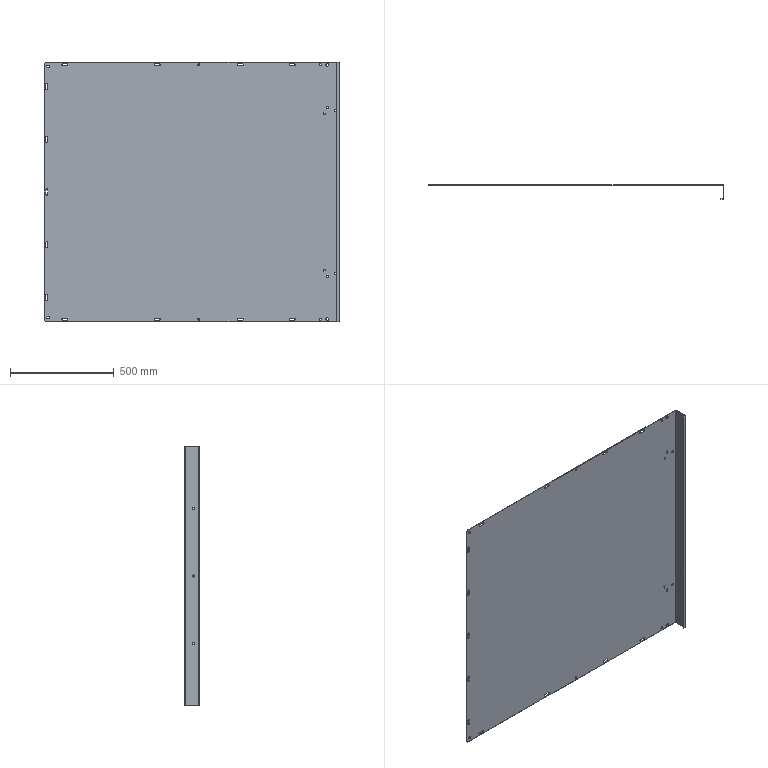Part | SolidWorks | features ICE 10, Cut 3, Fillet 1, FlatPattern 1, SMBaseFlange 1, SheetMetal 1 | 1 solid | 127 faces | box 1425 x 70 x 1250 mm | volume 5618902 mm3 | cylinder 67 | plane 60 | commonest cylinder face diameters 10 x39 10.5 x14 11 x4 12.8 x4 0.4 x2 6.4 x2